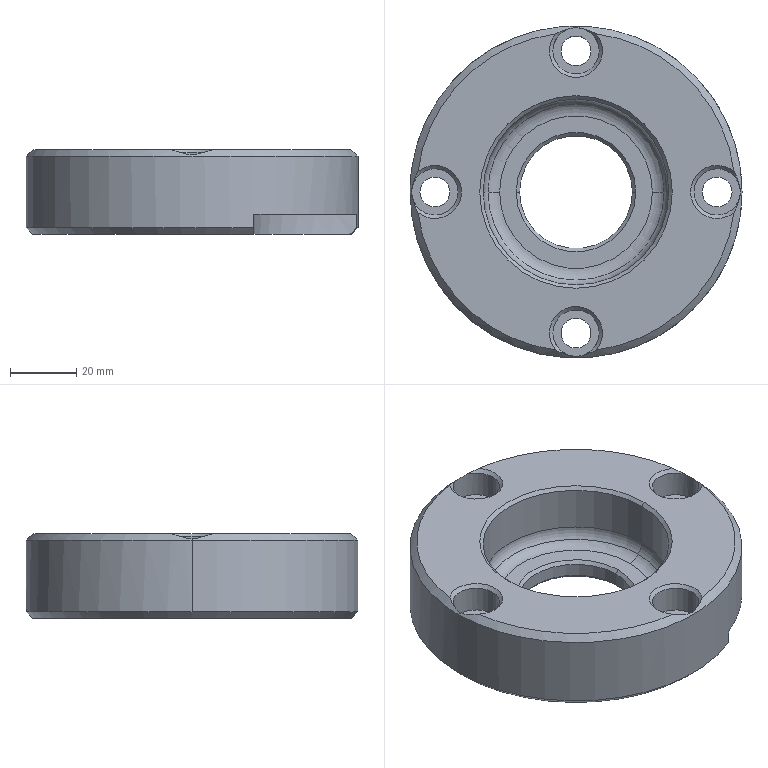Part | Creo | 1 solid | 59 faces | box 100 x 100 x 25.5 mm | volume 129793 mm3 | cylinder 24 | cone 22 | plane 9 | torus 4 | commonest cylinder face diameters 9 x8 14 x8 34 x2 56 x2 77 x2 100 x2